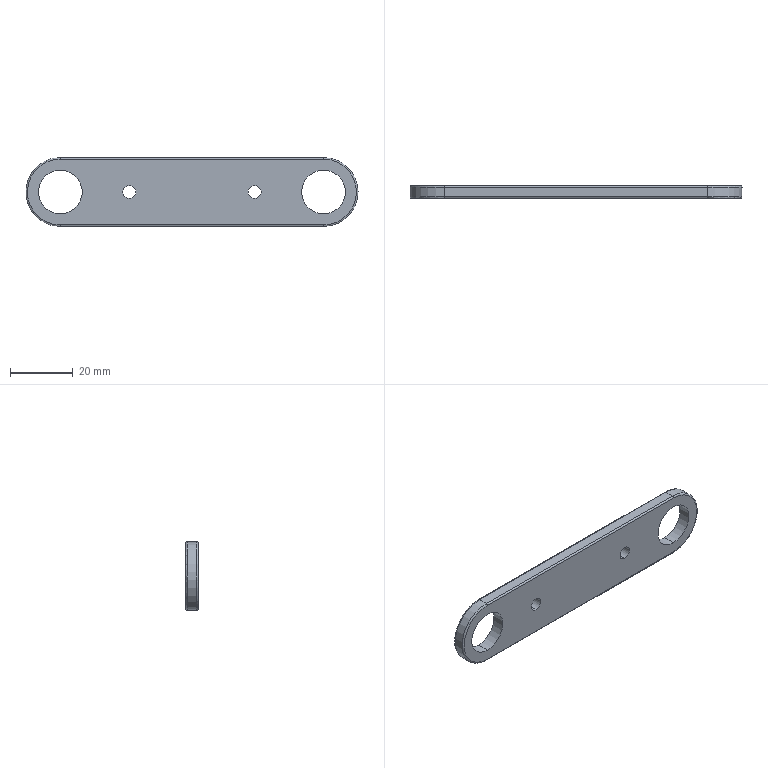Part | SolidWorks | features BaseBody 1 | 1 solid | 23 faces | box 106 x 4 x 22 mm | volume 7550 mm3 | cylinder 15 | plane 4 | spline 4 | commonest cylinder face diameters 1 x4 4.2 x4 13.97 x4 22 x3
STEP:
#1=CARTESIAN_POINT('',(42.,4.,-6.985));
#2=VERTEX_POINT('',#1);
#3=CARTESIAN_POINT('',(42.,4.,6.985));
#4=VERTEX_POINT('',#3);
#5=CARTESIAN_POINT('',(42.,4.,0.));
#6=DIRECTION('',(0.,1.,0.));
#7=DIRECTION('',(0.,0.,-1.));
#8=AXIS2_PLACEMENT_3D('',#5,#6,#7);
#9=CIRCLE('',#8,6.985);
#10=EDGE_CURVE('',#2,#4,#9,.T.);
#11=ORIENTED_EDGE('',*,*,#10,.T.);
#12=CARTESIAN_POINT('',(42.,0.,6.985));
#13=VERTEX_POINT('',#12);
#14=CARTESIAN_POINT('',(42.,4.,6.985));
#15=DIRECTION('',(0.,-1.,0.));
#16=VECTOR('',#15,1000.);
#17=LINE('',#14,#16);
#18=EDGE_CURVE('',#4,#13,#17,.T.);
#19=ORIENTED_EDGE('',*,*,#18,.T.);
#20=CARTESIAN_POINT('',(42.,0.,-6.985));
#21=VERTEX_POINT('',#20);
#22=CARTESIAN_POINT('',(42.,0.,0.));
#23=DIRECTION('',(0.,-1.,0.));
#24=DIRECTION('',(0.,0.,-1.));
#25=AXIS2_PLACEMENT_3D('',#22,#23,#24);
#26=CIRCLE('',#25,6.985);
#27=EDGE_CURVE('',#13,#21,#26,.T.);
#28=ORIENTED_EDGE('',*,*,#27,.T.);
#29=CARTESIAN_POINT('',(42.,4.,-6.985));
#30=DIRECTION('',(0.,-1.,0.));
#31=VECTOR('',#30,1000.);
#32=LINE('',#29,#31);
#33=EDGE_CURVE('',#2,#21,#32,.T.);
#34=ORIENTED_EDGE('',*,*,#33,.F.);
#35=EDGE_LOOP('',(#11,#19,#28,#34));
#36=FACE_OUTER_BOUND('',#35,.T.);
#37=CARTESIAN_POINT('',(42.,4.,0.));
#38=DIRECTION('',(0.,-1.,0.));
#39=DIRECTION('',(0.,0.,-1.));
#40=AXIS2_PLACEMENT_3D('',#37,#38,#39);
#41=CYLINDRICAL_SURFACE('',#40,6.985);
#42=ADVANCED_FACE('',(#36),#41,.F.);
#43=CARTESIAN_POINT('',(-42.,4.,6.985));
#44=VERTEX_POINT('',#43);
#45=CARTESIAN_POINT('',(-42.,4.,-6.985));
#46=VERTEX_POINT('',#45);
#47=CARTESIAN_POINT('',(-42.,4.,0.));
#48=DIRECTION('',(0.,-1.,0.));
#49=DIRECTION('',(0.,0.,-1.));
#50=AXIS2_PLACEMENT_3D('',#47,#48,#49);
#51=CIRCLE('',#50,6.985);
#52=EDGE_CURVE('',#44,#46,#51,.T.);
#53=ORIENTED_EDGE('',*,*,#52,.F.);
#54=CARTESIAN_POINT('',(-42.,0.,6.985));
#55=VERTEX_POINT('',#54);
#56=CARTESIAN_POINT('',(-42.,4.,6.985));
#57=DIRECTION('',(0.,-1.,0.));
#58=VECTOR('',#57,1000.);
#59=LINE('',#56,#58);
#60=EDGE_CURVE('',#44,#55,#59,.T.);
#61=ORIENTED_EDGE('',*,*,#60,.T.);
#62=CARTESIAN_POINT('',(-42.,0.,-6.985));
#63=VERTEX_POINT('',#62);
#64=CARTESIAN_POINT('',(-42.,0.,0.));
#65=DIRECTION('',(0.,-1.,0.));
#66=DIRECTION('',(0.,0.,-1.));
#67=AXIS2_PLACEMENT_3D('',#64,#65,#66);
#68=CIRCLE('',#67,6.985);
#69=EDGE_CURVE('',#55,#63,#68,.T.);
#70=ORIENTED_EDGE('',*,*,#69,.T.);
#71=CARTESIAN_POINT('',(-42.,4.,-6.985));
#72=DIRECTION('',(0.,-1.,0.));
#73=VECTOR('',#72,1000.);
#74=LINE('',#71,#73);
#75=EDGE_CURVE('',#46,#63,#74,.T.);
#76=ORIENTED_EDGE('',*,*,#75,.F.);
#77=EDGE_LOOP('',(#53,#61,#70,#76));
#78=FACE_OUTER_BOUND('',#77,.T.);
#79=CARTESIAN_POINT('',(-42.,4.,0.));
#80=DIRECTION('',(0.,-1.,0.));
#81=DIRECTION('',(0.,0.,-1.));
#82=AXIS2_PLACEMENT_3D('',#79,#80,#81);
#83=CYLINDRICAL_SURFACE('',#82,6.985);
#84=ADVANCED_FACE('',(#78),#83,.F.);
#85=CARTESIAN_POINT('',(-20.,4.,2.1));
#86=VERTEX_POINT('',#85);
#87=CARTESIAN_POINT('',(-20.,4.,-2.1));
#88=VERTEX_POINT('',#87);
#89=CARTESIAN_POINT('',(-20.,4.,0.));
#90=DIRECTION('',(0.,-1.,0.));
#91=DIRECTION('',(0.,0.,-1.));
#92=AXIS2_PLACEMENT_3D('',#89,#90,#91);
#93=CIRCLE('',#92,2.1);
#94=EDGE_CURVE('',#86,#88,#93,.T.);
#95=ORIENTED_EDGE('',*,*,#94,.F.);
#96=CARTESIAN_POINT('',(-20.,0.,2.1));
#97=VERTEX_POINT('',#96);
#98=CARTESIAN_POINT('',(-20.,4.,2.1));
#99=DIRECTION('',(0.,-1.,0.));
#100=VECTOR('',#99,1000.);
#101=LINE('',#98,#100);
#102=EDGE_CURVE('',#86,#97,#101,.T.);
#103=ORIENTED_EDGE('',*,*,#102,.T.);
#104=CARTESIAN_POINT('',(-20.,0.,-2.1));
#105=VERTEX_POINT('',#104);
#106=CARTESIAN_POINT('',(-20.,0.,0.));
#107=DIRECTION('',(0.,-1.,0.));
#108=DIRECTION('',(0.,0.,-1.));
#109=AXIS2_PLACEMENT_3D('',#106,#107,#108);
#110=CIRCLE('',#109,2.1);
#111=EDGE_CURVE('',#97,#105,#110,.T.);
#112=ORIENTED_EDGE('',*,*,#111,.T.);
#113=CARTESIAN_POINT('',(-20.,4.,-2.1));
#114=DIRECTION('',(0.,-1.,0.));
#115=VECTOR('',#114,1000.);
#116=LINE('',#113,#115);
#117=EDGE_CURVE('',#88,#105,#116,.T.);
#118=ORIENTED_EDGE('',*,*,#117,.F.);
#119=EDGE_LOOP('',(#95,#103,#112,#118));
#120=FACE_OUTER_BOUND('',#119,.T.);
#121=CARTESIAN_POINT('',(-20.,4.,0.));
#122=DIRECTION('',(0.,-1.,0.));
#123=DIRECTION('',(0.,0.,-1.));
#124=AXIS2_PLACEMENT_3D('',#121,#122,#123);
#125=CYLINDRICAL_SURFACE('',#124,2.1);
#126=ADVANCED_FACE('',(#120),#125,.F.);
#127=CARTESIAN_POINT('',(20.,4.,2.1));
#128=VERTEX_POINT('',#127);
#129=CARTESIAN_POINT('',(20.,4.,-2.1));
#130=VERTEX_POINT('',#129);
#131=CARTESIAN_POINT('',(20.,4.,0.));
#132=DIRECTION('',(0.,-1.,0.));
#133=DIRECTION('',(0.,0.,-1.));
#134=AXIS2_PLACEMENT_3D('',#131,#132,#133);
#135=CIRCLE('',#134,2.1);
#136=EDGE_CURVE('',#128,#130,#135,.T.);
#137=ORIENTED_EDGE('',*,*,#136,.F.);
#138=CARTESIAN_POINT('',(20.,0.,2.1));
#139=VERTEX_POINT('',#138);
#140=CARTESIAN_POINT('',(20.,4.,2.1));
#141=DIRECTION('',(0.,-1.,0.));
#142=VECTOR('',#141,1000.);
#143=LINE('',#140,#142);
#144=EDGE_CURVE('',#128,#139,#143,.T.);
#145=ORIENTED_EDGE('',*,*,#144,.T.);
#146=CARTESIAN_POINT('',(20.,0.,-2.1));
#147=VERTEX_POINT('',#146);
#148=CARTESIAN_POINT('',(20.,0.,0.));
#149=DIRECTION('',(0.,-1.,0.));
#150=DIRECTION('',(0.,0.,-1.));
#151=AXIS2_PLACEMENT_3D('',#148,#149,#150);
#152=CIRCLE('',#151,2.1);
#153=EDGE_CURVE('',#139,#147,#152,.T.);
#154=ORIENTED_EDGE('',*,*,#153,.T.);
#155=CARTESIAN_POINT('',(20.,4.,-2.1));
#156=DIRECTION('',(0.,-1.,0.));
#157=VECTOR('',#156,1000.);
#158=LINE('',#155,#157);
#159=EDGE_CURVE('',#130,#147,#158,.T.);
#160=ORIENTED_EDGE('',*,*,#159,.F.);
#161=EDGE_LOOP('',(#137,#145,#154,#160));
#162=FACE_OUTER_BOUND('',#161,.T.);
#163=CARTESIAN_POINT('',(20.,4.,0.));
#164=DIRECTION('',(0.,-1.,0.));
#165=DIRECTION('',(0.,0.,-1.));
#166=AXIS2_PLACEMENT_3D('',#163,#164,#165);
#167=CYLINDRICAL_SURFACE('',#166,2.1);
#168=ADVANCED_FACE('',(#162),#167,.F.);
#169=CARTESIAN_POINT('',(53.,3.5,0.));
#170=VERTEX_POINT('',#169);
#171=CARTESIAN_POINT('',(42.,3.5,-11.));
#172=VERTEX_POINT('',#171);
#173=CARTESIAN_POINT('',(42.,3.5,0.));
#174=DIRECTION('',(0.,1.,0.));
#175=DIRECTION('',(0.,0.,1.));
#176=AXIS2_PLACEMENT_3D('',#173,#174,#175);
#177=CIRCLE('',#176,11.);
#178=EDGE_CURVE('',#170,#172,#177,.T.);
#179=ORIENTED_EDGE('',*,*,#178,.F.);
#180=CARTESIAN_POINT('',(53.,0.5,0.));
#181=VERTEX_POINT('',#180);
#182=CARTESIAN_POINT('',(53.,3.5,0.));
#183=DIRECTION('',(0.,-1.,0.));
#184=VECTOR('',#183,1000.);
#185=LINE('',#182,#184);
#186=EDGE_CURVE('',#170,#181,#185,.T.);
#187=ORIENTED_EDGE('',*,*,#186,.T.);
#188=CARTESIAN_POINT('',(42.,0.5,-11.));
#189=VERTEX_POINT('',#188);
#190=CARTESIAN_POINT('',(42.,0.5,0.));
#191=DIRECTION('',(0.,-1.,0.));
#192=DIRECTION('',(0.,0.,-1.));
#193=AXIS2_PLACEMENT_3D('',#190,#191,#192);
#194=CIRCLE('',#193,11.);
#195=EDGE_CURVE('',#189,#181,#194,.T.);
#196=ORIENTED_EDGE('',*,*,#195,.F.);
#197=CARTESIAN_POINT('',(42.,2.,-11.));
#198=DIRECTION('',(0.,1.,0.));
#199=VECTOR('',#198,1000.);
#200=LINE('',#197,#199);
#201=EDGE_CURVE('',#189,#172,#200,.T.);
#202=ORIENTED_EDGE('',*,*,#201,.T.);
#203=EDGE_LOOP('',(#179,#187,#196,#202));
#204=FACE_OUTER_BOUND('',#203,.T.);
#205=CARTESIAN_POINT('',(42.,3.5,0.));
#206=DIRECTION('',(0.,-1.,0.));
#207=DIRECTION('',(1.,0.,0.));
#208=AXIS2_PLACEMENT_3D('',#205,#206,#207);
#209=CYLINDRICAL_SURFACE('',#208,11.);
#210=ADVANCED_FACE('',(#204),#209,.T.);
#211=ORIENTED_EDGE('',*,*,#18,.F.);
#212=CARTESIAN_POINT('',(42.,4.,0.));
#213=DIRECTION('',(0.,1.,0.));
#214=DIRECTION('',(0.,0.,-1.));
#215=AXIS2_PLACEMENT_3D('',#212,#213,#214);
#216=CIRCLE('',#215,6.985);
#217=EDGE_CURVE('',#4,#2,#216,.T.);
#218=ORIENTED_EDGE('',*,*,#217,.T.);
#219=ORIENTED_EDGE('',*,*,#33,.T.);
#220=CARTESIAN_POINT('',(42.,0.,0.));
#221=DIRECTION('',(0.,-1.,0.));
#222=DIRECTION('',(0.,0.,-1.));
#223=AXIS2_PLACEMENT_3D('',#220,#221,#222);
#224=CIRCLE('',#223,6.985);
#225=EDGE_CURVE('',#21,#13,#224,.T.);
#226=ORIENTED_EDGE('',*,*,#225,.T.);
#227=EDGE_LOOP('',(#211,#218,#219,#226));
#228=FACE_OUTER_BOUND('',#227,.T.);
#229=CARTESIAN_POINT('',(42.,4.,0.));
#230=DIRECTION('',(0.,-1.,0.));
#231=DIRECTION('',(0.,0.,-1.));
#232=AXIS2_PLACEMENT_3D('',#229,#230,#231);
#233=CYLINDRICAL_SURFACE('',#232,6.985);
#234=ADVANCED_FACE('',(#228),#233,.F.);
#235=ORIENTED_EDGE('',*,*,#225,.F.);
#236=ORIENTED_EDGE('',*,*,#27,.F.);
#237=EDGE_LOOP('',(#235,#236));
#238=FACE_BOUND('',#237,.T.);
#239=CARTESIAN_POINT('',(-42.,0.,0.));
#240=DIRECTION('',(0.,-1.,0.));
#241=DIRECTION('',(0.,0.,-1.));
#242=AXIS2_PLACEMENT_3D('',#239,#240,#241);
#243=CIRCLE('',#242,6.985);
#244=EDGE_CURVE('',#63,#55,#243,.T.);
#245=ORIENTED_EDGE('',*,*,#244,.F.);
#246=ORIENTED_EDGE('',*,*,#69,.F.);
#247=EDGE_LOOP('',(#245,#246));
#248=FACE_BOUND('',#247,.T.);
#249=CARTESIAN_POINT('',(-20.,0.,0.));
#250=DIRECTION('',(0.,-1.,0.));
#251=DIRECTION('',(0.,0.,-1.));
#252=AXIS2_PLACEMENT_3D('',#249,#250,#251);
#253=CIRCLE('',#252,2.1);
#254=EDGE_CURVE('',#105,#97,#253,.T.);
#255=ORIENTED_EDGE('',*,*,#254,.F.);
#256=ORIENTED_EDGE('',*,*,#111,.F.);
#257=EDGE_LOOP('',(#255,#256));
#258=FACE_BOUND('',#257,.T.);
#259=CARTESIAN_POINT('',(20.,0.,0.));
#260=DIRECTION('',(0.,-1.,0.));
#261=DIRECTION('',(0.,0.,-1.));
#262=AXIS2_PLACEMENT_3D('',#259,#260,#261);
#263=CIRCLE('',#262,2.1);
#264=EDGE_CURVE('',#147,#139,#263,.T.);
#265=ORIENTED_EDGE('',*,*,#264,.F.);
#266=ORIENTED_EDGE('',*,*,#153,.F.);
#267=EDGE_LOOP('',(#265,#266));
#268=FACE_BOUND('',#267,.T.);
#269=CARTESIAN_POINT('',(-42.,0.,-10.5));
#270=VERTEX_POINT('',#269);
#271=CARTESIAN_POINT('',(-42.,0.,10.5));
#272=VERTEX_POINT('',#271);
#273=CARTESIAN_POINT('',(-42.,0.,-10.5));
#274=CARTESIAN_POINT('',(-63.,0.,-10.5));
#275=CARTESIAN_POINT('',(-63.,0.,10.5));
#276=CARTESIAN_POINT('',(-42.,0.,10.5));
#277=(BOUNDED_CURVE()B_SPLINE_CURVE(3,(#273,#274,#275,#276),.UNSPECIFIED.,.F.,.T.)B_SPLINE_CURVE_WITH_KNOTS((4,4),(0.,1.),.UNSPECIFIED.)CURVE()GEOMETRIC_REPRESENTATION_ITEM()RATIONAL_B_SPLINE_CURVE((0.9566,0.3189,0.3189,0.9566))REPRESENTATION_ITEM(''));
#278=EDGE_CURVE('',#270,#272,#277,.T.);
#279=ORIENTED_EDGE('',*,*,#278,.F.);
#280=CARTESIAN_POINT('',(42.,0.,-10.5));
#281=VERTEX_POINT('',#280);
#282=CARTESIAN_POINT('',(0.,0.,-10.5));
#283=DIRECTION('',(-1.,0.,0.));
#284=VECTOR('',#283,1000.);
#285=LINE('',#282,#284);
#286=EDGE_CURVE('',#281,#270,#285,.T.);
#287=ORIENTED_EDGE('',*,*,#286,.F.);
#288=CARTESIAN_POINT('',(42.,0.,10.5));
#289=VERTEX_POINT('',#288);
#290=CARTESIAN_POINT('',(42.,0.,10.5));
#291=CARTESIAN_POINT('',(63.,0.,10.5));
#292=CARTESIAN_POINT('',(63.,0.,-10.5));
#293=CARTESIAN_POINT('',(42.,0.,-10.5));
#294=(BOUNDED_CURVE()B_SPLINE_CURVE(3,(#290,#291,#292,#293),.UNSPECIFIED.,.F.,.F.)B_SPLINE_CURVE_WITH_KNOTS((4,4),(0.,1.),.UNSPECIFIED.)CURVE()GEOMETRIC_REPRESENTATION_ITEM()RATIONAL_B_SPLINE_CURVE((0.9566,0.3189,0.3189,0.9566))REPRESENTATION_ITEM(''));
#295=EDGE_CURVE('',#289,#281,#294,.T.);
#296=ORIENTED_EDGE('',*,*,#295,.F.);
#297=CARTESIAN_POINT('',(0.,0.,10.5));
#298=DIRECTION('',(1.,0.,0.));
#299=VECTOR('',#298,1000.);
#300=LINE('',#297,#299);
#301=EDGE_CURVE('',#272,#289,#300,.T.);
#302=ORIENTED_EDGE('',*,*,#301,.F.);
#303=EDGE_LOOP('',(#279,#287,#296,#302));
#304=FACE_OUTER_BOUND('',#303,.T.);
#305=CARTESIAN_POINT('',(-53.13,0.,-10.5));
#306=DIRECTION('',(0.,1.,0.));
#307=DIRECTION('',(0.,0.,1.));
#308=AXIS2_PLACEMENT_3D('',#305,#306,#307);
#309=PLANE('',#308);
#310=ADVANCED_FACE('',(#238,#248,#258,#268,#304),#309,.F.);
#311=ORIENTED_EDGE('',*,*,#10,.F.);
#312=ORIENTED_EDGE('',*,*,#217,.F.);
#313=EDGE_LOOP('',(#311,#312));
#314=FACE_BOUND('',#313,.T.);
#315=CARTESIAN_POINT('',(-42.,4.,0.));
#316=DIRECTION('',(0.,-1.,0.));
#317=DIRECTION('',(0.,0.,-1.));
#318=AXIS2_PLACEMENT_3D('',#315,#316,#317);
#319=CIRCLE('',#318,6.985);
#320=EDGE_CURVE('',#46,#44,#319,.T.);
#321=ORIENTED_EDGE('',*,*,#320,.T.);
#322=ORIENTED_EDGE('',*,*,#52,.T.);
#323=EDGE_LOOP('',(#321,#322));
#324=FACE_BOUND('',#323,.T.);
#325=CARTESIAN_POINT('',(-20.,4.,0.));
#326=DIRECTION('',(0.,-1.,0.));
#327=DIRECTION('',(0.,0.,-1.));
#328=AXIS2_PLACEMENT_3D('',#325,#326,#327);
#329=CIRCLE('',#328,2.1);
#330=EDGE_CURVE('',#88,#86,#329,.T.);
#331=ORIENTED_EDGE('',*,*,#330,.T.);
#332=ORIENTED_EDGE('',*,*,#94,.T.);
#333=EDGE_LOOP('',(#331,#332));
#334=FACE_BOUND('',#333,.T.);
#335=CARTESIAN_POINT('',(20.,4.,0.));
#336=DIRECTION('',(0.,-1.,0.));
#337=DIRECTION('',(0.,0.,-1.));
#338=AXIS2_PLACEMENT_3D('',#335,#336,#337);
#339=CIRCLE('',#338,2.1);
#340=EDGE_CURVE('',#130,#128,#339,.T.);
#341=ORIENTED_EDGE('',*,*,#340,.T.);
#342=ORIENTED_EDGE('',*,*,#136,.T.);
#343=EDGE_LOOP('',(#341,#342));
#344=FACE_BOUND('',#343,.T.);
#345=CARTESIAN_POINT('',(-42.,4.,10.5));
#346=VERTEX_POINT('',#345);
#347=CARTESIAN_POINT('',(42.,4.,10.5));
#348=VERTEX_POINT('',#347);
#349=CARTESIAN_POINT('',(0.,4.,10.5));
#350=DIRECTION('',(1.,0.,0.));
#351=VECTOR('',#350,1000.);
#352=LINE('',#349,#351);
#353=EDGE_CURVE('',#346,#348,#352,.T.);
#354=ORIENTED_EDGE('',*,*,#353,.T.);
#355=CARTESIAN_POINT('',(42.,4.,-10.5));
#356=VERTEX_POINT('',#355);
#357=CARTESIAN_POINT('',(42.,4.,10.5));
#358=CARTESIAN_POINT('',(42.233,4.,10.5));
#359=CARTESIAN_POINT('',(42.583,4.,10.488));
#360=CARTESIAN_POINT('',(42.989,4.,10.454));
#361=CARTESIAN_POINT('',(43.191,4.,10.432));
#362=CARTESIAN_POINT('',(43.293,4.,10.42));
#363=CARTESIAN_POINT('',(43.336,4.,10.415));
#364=CARTESIAN_POINT('',(43.365,4.,10.411));
#365=CARTESIAN_POINT('',(43.377,4.,10.409));
#366=CARTESIAN_POINT('',(43.655,4.,10.372));
#367=CARTESIAN_POINT('',(44.045,4.,10.305));
#368=CARTESIAN_POINT('',(44.494,4.,10.201));
#369=CARTESIAN_POINT('',(44.718,4.,10.143));
#370=CARTESIAN_POINT('',(44.829,4.,10.112));
#371=CARTESIAN_POINT('',(44.877,4.,10.098));
#372=CARTESIAN_POINT('',(44.908,4.,10.089));
#373=CARTESIAN_POINT('',(44.922,4.,10.085));
#374=CARTESIAN_POINT('',(45.226,4.,9.997));
#375=CARTESIAN_POINT('',(45.648,4.,9.854));
#376=CARTESIAN_POINT('',(46.128,4.,9.656));
#377=CARTESIAN_POINT('',(46.366,4.,9.55));
#378=CARTESIAN_POINT('',(46.484,4.,9.495));
#379=CARTESIAN_POINT('',(46.534,4.,9.471));
#380=CARTESIAN_POINT('',(46.568,4.,9.454));
#381=CARTESIAN_POINT('',(46.582,4.,9.447));
#382=CARTESIAN_POINT('',(46.901,4.,9.292));
#383=CARTESIAN_POINT('',(47.338,4.,9.053));
#384=CARTESIAN_POINT('',(47.826,4.,8.738));
#385=CARTESIAN_POINT('',(48.065,4.,8.572));
#386=CARTESIAN_POINT('',(48.183,4.,8.487));
#387=CARTESIAN_POINT('',(48.233,4.,8.45));
#388=CARTESIAN_POINT('',(48.267,4.,8.425));
#389=CARTESIAN_POINT('',(48.282,4.,8.414));
#390=CARTESIAN_POINT('',(48.595,4.,8.179));
#391=CARTESIAN_POINT('',(49.017,4.,7.826));
#392=CARTESIAN_POINT('',(49.475,4.,7.378));
#393=CARTESIAN_POINT('',(49.696,4.,7.144));
#394=CARTESIAN_POINT('',(49.804,4.,7.025));
#395=CARTESIAN_POINT('',(49.85,4.,6.973));
#396=CARTESIAN_POINT('',(49.881,4.,6.939));
#397=CARTESIAN_POINT('',(49.895,4.,6.923));
#398=CARTESIAN_POINT('',(50.04,4.,6.757));
#399=CARTESIAN_POINT('',(50.226,4.,6.53));
#400=CARTESIAN_POINT('',(50.433,4.,6.258));
#401=CARTESIAN_POINT('',(50.519,4.,6.139));
#402=CARTESIAN_POINT('',(50.576,4.,6.059));
#403=CARTESIAN_POINT('',(50.603,4.,6.02));
#404=CARTESIAN_POINT('',(50.747,4.,5.812));
#405=CARTESIAN_POINT('',(50.913,4.,5.557));
#406=CARTESIAN_POINT('',(51.093,4.,5.252));
#407=CARTESIAN_POINT('',(51.168,4.,5.119));
#408=CARTESIAN_POINT('',(51.217,4.,5.031));
#409=CARTESIAN_POINT('',(51.24,4.,4.987));
#410=CARTESIAN_POINT('',(51.363,4.,4.757));
#411=CARTESIAN_POINT('',(51.502,4.,4.477));
#412=CARTESIAN_POINT('',(51.628,4.,4.19));
#413=CARTESIAN_POINT('',(51.71,4.,3.998));
#414=CARTESIAN_POINT('',(51.748,4.,3.903));
#415=CARTESIAN_POINT('',(51.864,4.,3.605));
#416=CARTESIAN_POINT('',(51.971,4.,3.303));
#417=CARTESIAN_POINT('',(52.064,4.,2.997));
#418=CARTESIAN_POINT('',(52.123,4.,2.791));
#419=CARTESIAN_POINT('',(52.15,4.,2.69));
#420=CARTESIAN_POINT('',(52.23,4.,2.374));
#421=CARTESIAN_POINT('',(52.277,4.,2.163));
#422=CARTESIAN_POINT('',(52.358,4.,1.737));
#423=CARTESIAN_POINT('',(52.391,4.,1.524));
#424=CARTESIAN_POINT('',(52.473,4.,0.8737));
#425=CARTESIAN_POINT('',(52.5,4.,0.4371));
#426=CARTESIAN_POINT('',(52.5,4.,-0.2186));
#427=CARTESIAN_POINT('',(52.493,4.,-0.4368));
#428=CARTESIAN_POINT('',(52.466,4.,-0.8726));
#429=CARTESIAN_POINT('',(52.445,4.,-1.092));
#430=CARTESIAN_POINT('',(52.391,4.,-1.523));
#431=CARTESIAN_POINT('',(52.341,4.,-1.844));
#432=CARTESIAN_POINT('',(52.276,4.,-2.162));
#433=CARTESIAN_POINT('',(52.229,4.,-2.374));
#434=CARTESIAN_POINT('',(52.203,4.,-2.481));
#435=CARTESIAN_POINT('',(52.124,4.,-2.792));
#436=CARTESIAN_POINT('',(52.036,4.,-3.099));
#437=CARTESIAN_POINT('',(51.917,4.,-3.453));
#438=CARTESIAN_POINT('',(51.862,4.,-3.604));
#439=CARTESIAN_POINT('',(51.825,4.,-3.704));
#440=CARTESIAN_POINT('',(51.806,4.,-3.755));
#441=CARTESIAN_POINT('',(51.711,4.,-3.998));
#442=CARTESIAN_POINT('',(51.589,4.,-4.287));
#443=CARTESIAN_POINT('',(51.432,4.,-4.616));
#444=CARTESIAN_POINT('',(51.361,4.,-4.756));
#445=CARTESIAN_POINT('',(51.314,4.,-4.849));
#446=CARTESIAN_POINT('',(51.289,4.,-4.896));
#447=CARTESIAN_POINT('',(51.169,4.,-5.12));
#448=CARTESIAN_POINT('',(51.019,4.,-5.384));
#449=CARTESIAN_POINT('',(50.83,4.,-5.684));
#450=CARTESIAN_POINT('',(50.746,4.,-5.811));
#451=CARTESIAN_POINT('',(50.689,4.,-5.895));
#452=CARTESIAN_POINT('',(50.66,4.,-5.938));
#453=CARTESIAN_POINT('',(50.52,4.,-6.139));
#454=CARTESIAN_POINT('',(50.347,4.,-6.376));
#455=CARTESIAN_POINT('',(50.133,4.,-6.643));
#456=CARTESIAN_POINT('',(50.023,4.,-6.774));
#457=CARTESIAN_POINT('',(49.975,4.,-6.83));
#458=CARTESIAN_POINT('',(49.943,4.,-6.867));
#459=CARTESIAN_POINT('',(49.926,4.,-6.887));
#460=CARTESIAN_POINT('',(49.669,4.,-7.182));
#461=CARTESIAN_POINT('',(49.286,4.,-7.577));
#462=CARTESIAN_POINT('',(48.804,4.,-8.001));
#463=CARTESIAN_POINT('',(48.555,4.,-8.203));
#464=CARTESIAN_POINT('',(48.428,4.,-8.302));
#465=CARTESIAN_POINT('',(48.373,4.,-8.344));
#466=CARTESIAN_POINT('',(48.337,4.,-8.372));
#467=CARTESIAN_POINT('',(48.317,4.,-8.388));
#468=CARTESIAN_POINT('',(48.033,4.,-8.6));
#469=CARTESIAN_POINT('',(47.621,4.,-8.88));
#470=CARTESIAN_POINT('',(47.118,4.,-9.171));
#471=CARTESIAN_POINT('',(46.862,4.,-9.307));
#472=CARTESIAN_POINT('',(46.732,4.,-9.374));
#473=CARTESIAN_POINT('',(46.676,4.,-9.401));
#474=CARTESIAN_POINT('',(46.639,4.,-9.42));
#475=CARTESIAN_POINT('',(46.618,4.,-9.43));
#476=CARTESIAN_POINT('',(46.334,4.,-9.569));
#477=CARTESIAN_POINT('',(45.925,4.,-9.747));
#478=CARTESIAN_POINT('',(45.437,4.,-9.924));
#479=CARTESIAN_POINT('',(45.189,4.,-10.004));
#480=CARTESIAN_POINT('',(45.065,4.,-10.043));
#481=CARTESIAN_POINT('',(45.011,4.,-10.059));
#482=CARTESIAN_POINT('',(44.976,4.,-10.07));
#483=CARTESIAN_POINT('',(44.956,4.,-10.075));
#484=CARTESIAN_POINT('',(44.687,4.,-10.154));
#485=CARTESIAN_POINT('',(44.303,4.,-10.25));
#486=CARTESIAN_POINT('',(43.85,4.,-10.337));
#487=CARTESIAN_POINT('',(43.623,4.,-10.374));
#488=CARTESIAN_POINT('',(43.508,4.,-10.391));
#489=CARTESIAN_POINT('',(43.459,4.,-10.398));
#490=CARTESIAN_POINT('',(43.427,4.,-10.403));
#491=CARTESIAN_POINT('',(43.408,4.,-10.405));
#492=CARTESIAN_POINT('',(42.932,4.,-10.469));
#493=CARTESIAN_POINT('',(42.467,4.,-10.5));
#494=CARTESIAN_POINT('',(42.,4.,-10.5));
#495=B_SPLINE_CURVE_WITH_KNOTS('',3,(#357,#358,#359,#360,#361,#362,#363,#364,#365,#366,#367,#368,#369,#370,#371,#372,#373,#374,#375,#376,#377,#378,#379,#380,#381,#382,#383,#384,#385,#386,#387,#388,#389,#390,#391,#392,#393,#394,#395,#396,#397,#398,#399,#400,#401,#402,#403,#404,#405,#406,#407,#408,#409,#410,#411,#412,#413,#414,#415,#416,#417,#418,#419,#420,#421,#422,#423,#424,#425,#426,#427,#428,#429,#430,#431,#432,#433,#434,#435,#436,#437,#438,#439,#440,#441,#442,#443,#444,#445,#446,#447,#448,#449,#450,#451,#452,#453,#454,#455,#456,#457,#458,#459,#460,#461,#462,#463,#464,#465,#466,#467,#468,#469,#470,#471,#472,#473,#474,#475,#476,#477,#478,#479,#480,#481,#482,#483,#484,#485,#486,#487,#488,#489,#490,#491,#492,#493,#494),.UNSPECIFIED.,.F.,.F.,(4,1,1,1,1,2,2,1,1,1,1,2,2,1,1,1,1,2,2,1,1,1,1,2,2,1,1,1,1,2,2,1,1,2,2,1,1,2,2,1,2,2,1,2,2,2,2,2,2,2,1,2,2,1,1,2,2,1,1,2,2,1,1,2,2,1,1,1,2,2,1,1,1,1,2,2,1,1,1,1,2,2,1,1,1,1,2,2,1,1,1,1,2,2,4),(0.,0.03125,0.04688,0.05469,0.05859,0.06055,0.0625,0.09375,0.1094,0.1172,0.1211,0.123,0.125,0.1563,0.1719,0.1797,0.1836,0.1855,0.1875,0.2188,0.2344,0.2422,0.2461,0.248,0.25,0.2813,0.2969,0.3047,0.3086,0.3105,0.3125,0.3281,0.3359,0.3398,0.3438,0.3594,0.3672,0.3711,0.375,0.3906,0.3984,0.4063,0.4219,0.4297,0.4375,0.4531,0.4688,0.5,0.5156,0.5313,0.5469,0.5547,0.5625,0.5781,0.5859,0.5898,0.5938,0.6094,0.6172,0.6211,0.625,0.6406,0.6484,0.6523,0.6562,0.6719,0.6797,0.6836,0.6855,0.6875,0.7187,0.7344,0.7422,0.7461,0.748,0.75,0.7812,0.7969,0.8047,0.8086,0.8105,0.8125,0.8437,0.8594,0.8672,0.8711,0.873,0.875,0.9062,0.9219,0.9297,0.9336,0.9355,0.9375,1.),.UNSPECIFIED.);
#496=EDGE_CURVE('',#348,#356,#495,.T.);
#497=ORIENTED_EDGE('',*,*,#496,.T.);
#498=CARTESIAN_POINT('',(-42.,4.,-10.5));
#499=VERTEX_POINT('',#498);
#500=CARTESIAN_POINT('',(0.,4.,-10.5));
#501=DIRECTION('',(-1.,0.,0.));
#502=VECTOR('',#501,1000.);
#503=LINE('',#500,#502);
#504=EDGE_CURVE('',#356,#499,#503,.T.);
#505=ORIENTED_EDGE('',*,*,#504,.T.);
#506=CARTESIAN_POINT('',(-42.,4.,-10.5));
#507=CARTESIAN_POINT('',(-42.233,4.,-10.5));
#508=CARTESIAN_POINT('',(-42.583,4.,-10.488));
#509=CARTESIAN_POINT('',(-42.989,4.,-10.454));
#510=CARTESIAN_POINT('',(-43.191,4.,-10.432));
#511=CARTESIAN_POINT('',(-43.293,4.,-10.42));
#512=CARTESIAN_POINT('',(-43.336,4.,-10.415));
#513=CARTESIAN_POINT('',(-43.365,4.,-10.411));
#514=CARTESIAN_POINT('',(-43.377,4.,-10.409));
#515=CARTESIAN_POINT('',(-43.655,4.,-10.372));
#516=CARTESIAN_POINT('',(-44.045,4.,-10.305));
#517=CARTESIAN_POINT('',(-44.494,4.,-10.201));
#518=CARTESIAN_POINT('',(-44.718,4.,-10.143));
#519=CARTESIAN_POINT('',(-44.829,4.,-10.112));
#520=CARTESIAN_POINT('',(-44.877,4.,-10.098));
#521=CARTESIAN_POINT('',(-44.908,4.,-10.089));
#522=CARTESIAN_POINT('',(-44.922,4.,-10.085));
#523=CARTESIAN_POINT('',(-45.226,4.,-9.997));
#524=CARTESIAN_POINT('',(-45.648,4.,-9.854));
#525=CARTESIAN_POINT('',(-46.128,4.,-9.656));
#526=CARTESIAN_POINT('',(-46.366,4.,-9.55));
#527=CARTESIAN_POINT('',(-46.484,4.,-9.495));
#528=CARTESIAN_POINT('',(-46.534,4.,-9.471));
#529=CARTESIAN_POINT('',(-46.568,4.,-9.454));
#530=CARTESIAN_POINT('',(-46.582,4.,-9.447));
#531=CARTESIAN_POINT('',(-46.901,4.,-9.292));
#532=CARTESIAN_POINT('',(-47.338,4.,-9.053));
#533=CARTESIAN_POINT('',(-47.826,4.,-8.738));
#534=CARTESIAN_POINT('',(-48.065,4.,-8.572));
#535=CARTESIAN_POINT('',(-48.183,4.,-8.487));
#536=CARTESIAN_POINT('',(-48.233,4.,-8.45));
#537=CARTESIAN_POINT('',(-48.267,4.,-8.425));
#538=CARTESIAN_POINT('',(-48.282,4.,-8.414));
#539=CARTESIAN_POINT('',(-48.595,4.,-8.179));
#540=CARTESIAN_POINT('',(-49.017,4.,-7.826));
#541=CARTESIAN_POINT('',(-49.475,4.,-7.378));
#542=CARTESIAN_POINT('',(-49.696,4.,-7.144));
#543=CARTESIAN_POINT('',(-49.804,4.,-7.025));
#544=CARTESIAN_POINT('',(-49.85,4.,-6.973));
#545=CARTESIAN_POINT('',(-49.881,4.,-6.939));
#546=CARTESIAN_POINT('',(-49.895,4.,-6.923));
#547=CARTESIAN_POINT('',(-50.04,4.,-6.757));
#548=CARTESIAN_POINT('',(-50.226,4.,-6.53));
#549=CARTESIAN_POINT('',(-50.433,4.,-6.258));
#550=CARTESIAN_POINT('',(-50.519,4.,-6.139));
#551=CARTESIAN_POINT('',(-50.576,4.,-6.059));
#552=CARTESIAN_POINT('',(-50.603,4.,-6.02));
#553=CARTESIAN_POINT('',(-50.747,4.,-5.812));
#554=CARTESIAN_POINT('',(-50.913,4.,-5.557));
#555=CARTESIAN_POINT('',(-51.093,4.,-5.252));
#556=CARTESIAN_POINT('',(-51.168,4.,-5.119));
#557=CARTESIAN_POINT('',(-51.217,4.,-5.031));
#558=CARTESIAN_POINT('',(-51.24,4.,-4.987));
#559=CARTESIAN_POINT('',(-51.363,4.,-4.757));
#560=CARTESIAN_POINT('',(-51.502,4.,-4.477));
#561=CARTESIAN_POINT('',(-51.628,4.,-4.19));
#562=CARTESIAN_POINT('',(-51.71,4.,-3.998));
#563=CARTESIAN_POINT('',(-51.748,4.,-3.903));
#564=CARTESIAN_POINT('',(-51.864,4.,-3.605));
#565=CARTESIAN_POINT('',(-51.971,4.,-3.303));
#566=CARTESIAN_POINT('',(-52.064,4.,-2.997));
#567=CARTESIAN_POINT('',(-52.123,4.,-2.791));
#568=CARTESIAN_POINT('',(-52.15,4.,-2.69));
#569=CARTESIAN_POINT('',(-52.23,4.,-2.374));
#570=CARTESIAN_POINT('',(-52.277,4.,-2.163));
#571=CARTESIAN_POINT('',(-52.358,4.,-1.737));
#572=CARTESIAN_POINT('',(-52.391,4.,-1.524));
#573=CARTESIAN_POINT('',(-52.473,4.,-0.8737));
#574=CARTESIAN_POINT('',(-52.5,4.,-0.4371));
#575=CARTESIAN_POINT('',(-52.5,4.,0.2186));
#576=CARTESIAN_POINT('',(-52.493,4.,0.4368));
#577=CARTESIAN_POINT('',(-52.466,4.,0.8726));
#578=CARTESIAN_POINT('',(-52.445,4.,1.092));
#579=CARTESIAN_POINT('',(-52.391,4.,1.523));
#580=CARTESIAN_POINT('',(-52.341,4.,1.844));
#581=CARTESIAN_POINT('',(-52.276,4.,2.162));
#582=CARTESIAN_POINT('',(-52.229,4.,2.374));
#583=CARTESIAN_POINT('',(-52.203,4.,2.481));
#584=CARTESIAN_POINT('',(-52.124,4.,2.792));
#585=CARTESIAN_POINT('',(-52.036,4.,3.099));
#586=CARTESIAN_POINT('',(-51.917,4.,3.453));
#587=CARTESIAN_POINT('',(-51.862,4.,3.604));
#588=CARTESIAN_POINT('',(-51.825,4.,3.704));
#589=CARTESIAN_POINT('',(-51.806,4.,3.755));
#590=CARTESIAN_POINT('',(-51.711,4.,3.998));
#591=CARTESIAN_POINT('',(-51.589,4.,4.287));
#592=CARTESIAN_POINT('',(-51.432,4.,4.616));
#593=CARTESIAN_POINT('',(-51.361,4.,4.756));
#594=CARTESIAN_POINT('',(-51.314,4.,4.849));
#595=CARTESIAN_POINT('',(-51.289,4.,4.896));
#596=CARTESIAN_POINT('',(-51.169,4.,5.12));
#597=CARTESIAN_POINT('',(-51.019,4.,5.384));
#598=CARTESIAN_POINT('',(-50.83,4.,5.684));
#599=CARTESIAN_POINT('',(-50.746,4.,5.811));
#600=CARTESIAN_POINT('',(-50.689,4.,5.895));
#601=CARTESIAN_POINT('',(-50.66,4.,5.938));
#602=CARTESIAN_POINT('',(-50.52,4.,6.139));
#603=CARTESIAN_POINT('',(-50.347,4.,6.376));
#604=CARTESIAN_POINT('',(-50.133,4.,6.643));
#605=CARTESIAN_POINT('',(-50.023,4.,6.774));
#606=CARTESIAN_POINT('',(-49.975,4.,6.83));
#607=CARTESIAN_POINT('',(-49.943,4.,6.867));
#608=CARTESIAN_POINT('',(-49.926,4.,6.887));
#609=CARTESIAN_POINT('',(-49.669,4.,7.182));
#610=CARTESIAN_POINT('',(-49.286,4.,7.577));
#611=CARTESIAN_POINT('',(-48.804,4.,8.001));
#612=CARTESIAN_POINT('',(-48.555,4.,8.203));
#613=CARTESIAN_POINT('',(-48.428,4.,8.302));
#614=CARTESIAN_POINT('',(-48.373,4.,8.344));
#615=CARTESIAN_POINT('',(-48.337,4.,8.372));
#616=CARTESIAN_POINT('',(-48.317,4.,8.388));
#617=CARTESIAN_POINT('',(-48.033,4.,8.6));
#618=CARTESIAN_POINT('',(-47.621,4.,8.88));
#619=CARTESIAN_POINT('',(-47.118,4.,9.171));
#620=CARTESIAN_POINT('',(-46.862,4.,9.307));
#621=CARTESIAN_POINT('',(-46.732,4.,9.374));
#622=CARTESIAN_POINT('',(-46.676,4.,9.401));
#623=CARTESIAN_POINT('',(-46.639,4.,9.42));
#624=CARTESIAN_POINT('',(-46.618,4.,9.43));
#625=CARTESIAN_POINT('',(-46.334,4.,9.569));
#626=CARTESIAN_POINT('',(-45.925,4.,9.747));
#627=CARTESIAN_POINT('',(-45.437,4.,9.924));
#628=CARTESIAN_POINT('',(-45.189,4.,10.004));
#629=CARTESIAN_POINT('',(-45.065,4.,10.043));
#630=CARTESIAN_POINT('',(-45.011,4.,10.059));
#631=CARTESIAN_POINT('',(-44.976,4.,10.07));
#632=CARTESIAN_POINT('',(-44.956,4.,10.075));
#633=CARTESIAN_POINT('',(-44.687,4.,10.154));
#634=CARTESIAN_POINT('',(-44.303,4.,10.25));
#635=CARTESIAN_POINT('',(-43.85,4.,10.337));
#636=CARTESIAN_POINT('',(-43.623,4.,10.374));
#637=CARTESIAN_POINT('',(-43.508,4.,10.391));
#638=CARTESIAN_POINT('',(-43.459,4.,10.398));
#639=CARTESIAN_POINT('',(-43.427,4.,10.403));
#640=CARTESIAN_POINT('',(-43.408,4.,10.405));
#641=CARTESIAN_POINT('',(-42.932,4.,10.469));
#642=CARTESIAN_POINT('',(-42.467,4.,10.5));
#643=CARTESIAN_POINT('',(-42.,4.,10.5));
#644=B_SPLINE_CURVE_WITH_KNOTS('',3,(#506,#507,#508,#509,#510,#511,#512,#513,#514,#515,#516,#517,#518,#519,#520,#521,#522,#523,#524,#525,#526,#527,#528,#529,#530,#531,#532,#533,#534,#535,#536,#537,#538,#539,#540,#541,#542,#543,#544,#545,#546,#547,#548,#549,#550,#551,#552,#553,#554,#555,#556,#557,#558,#559,#560,#561,#562,#563,#564,#565,#566,#567,#568,#569,#570,#571,#572,#573,#574,#575,#576,#577,#578,#579,#580,#581,#582,#583,#584,#585,#586,#587,#588,#589,#590,#591,#592,#593,#594,#595,#596,#597,#598,#599,#600,#601,#602,#603,#604,#605,#606,#607,#608,#609,#610,#611,#612,#613,#614,#615,#616,#617,#618,#619,#620,#621,#622,#623,#624,#625,#626,#627,#628,#629,#630,#631,#632,#633,#634,#635,#636,#637,#638,#639,#640,#641,#642,#643),.UNSPECIFIED.,.F.,.F.,(4,1,1,1,1,2,2,1,1,1,1,2,2,1,1,1,1,2,2,1,1,1,1,2,2,1,1,1,1,2,2,1,1,2,2,1,1,2,2,1,2,2,1,2,2,2,2,2,2,2,1,2,2,1,1,2,2,1,1,2,2,1,1,2,2,1,1,1,2,2,1,1,1,1,2,2,1,1,1,1,2,2,1,1,1,1,2,2,1,1,1,1,2,2,4),(0.,0.03125,0.04687,0.05469,0.05859,0.06055,0.0625,0.09375,0.1094,0.1172,0.1211,0.123,0.125,0.1562,0.1719,0.1797,0.1836,0.1855,0.1875,0.2187,0.2344,0.2422,0.2461,0.248,0.25,0.2812,0.2969,0.3047,0.3086,0.3105,0.3125,0.3281,0.3359,0.3398,0.3437,0.3594,0.3672,0.3711,0.375,0.3906,0.3984,0.4062,0.4219,0.4297,0.4375,0.4531,0.4687,0.5,0.5156,0.5312,0.5469,0.5547,0.5625,0.5781,0.5859,0.5898,0.5937,0.6094,0.6172,0.6211,0.625,0.6406,0.6484,0.6523,0.6562,0.6719,0.6797,0.6836,0.6855,0.6875,0.7187,0.7344,0.7422,0.7461,0.748,0.75,0.7812,0.7969,0.8047,0.8086,0.8105,0.8125,0.8437,0.8594,0.8672,0.8711,0.873,0.875,0.9062,0.9219,0.9297,0.9336,0.9355,0.9375,1.),.UNSPECIFIED.);
#645=EDGE_CURVE('',#499,#346,#644,.T.);
#646=ORIENTED_EDGE('',*,*,#645,.T.);
#647=EDGE_LOOP('',(#354,#497,#505,#646));
#648=FACE_OUTER_BOUND('',#647,.T.);
#649=CARTESIAN_POINT('',(-53.13,4.,-10.5));
#650=DIRECTION('',(0.,1.,0.));
#651=DIRECTION('',(0.,0.,1.));
#652=AXIS2_PLACEMENT_3D('',#649,#650,#651);
#653=PLANE('',#652);
#654=ADVANCED_FACE('',(#314,#324,#334,#344,#648),#653,.T.);
#655=ORIENTED_EDGE('',*,*,#60,.F.);
#656=ORIENTED_EDGE('',*,*,#320,.F.);
#657=ORIENTED_EDGE('',*,*,#75,.T.);
#658=ORIENTED_EDGE('',*,*,#244,.T.);
#659=EDGE_LOOP('',(#655,#656,#657,#658));
#660=FACE_OUTER_BOUND('',#659,.T.);
#661=CARTESIAN_POINT('',(-42.,4.,0.));
#662=DIRECTION('',(0.,-1.,0.));
#663=DIRECTION('',(0.,0.,-1.));
#664=AXIS2_PLACEMENT_3D('',#661,#662,#663);
#665=CYLINDRICAL_SURFACE('',#664,6.985);
#666=ADVANCED_FACE('',(#660),#665,.F.);
#667=ORIENTED_EDGE('',*,*,#102,.F.);
#668=ORIENTED_EDGE('',*,*,#330,.F.);
#669=ORIENTED_EDGE('',*,*,#117,.T.);
#670=ORIENTED_EDGE('',*,*,#254,.T.);
#671=EDGE_LOOP('',(#667,#668,#669,#670));
#672=FACE_OUTER_BOUND('',#671,.T.);
#673=CARTESIAN_POINT('',(-20.,4.,0.));
#674=DIRECTION('',(0.,-1.,0.));
#675=DIRECTION('',(0.,0.,-1.));
#676=AXIS2_PLACEMENT_3D('',#673,#674,#675);
#677=CYLINDRICAL_SURFACE('',#676,2.1);
#678=ADVANCED_FACE('',(#672),#677,.F.);
#679=ORIENTED_EDGE('',*,*,#144,.F.);
#680=ORIENTED_EDGE('',*,*,#340,.F.);
#681=ORIENTED_EDGE('',*,*,#159,.T.);
#682=ORIENTED_EDGE('',*,*,#264,.T.);
#683=EDGE_LOOP('',(#679,#680,#681,#682));
#684=FACE_OUTER_BOUND('',#683,.T.);
#685=CARTESIAN_POINT('',(20.,4.,0.));
#686=DIRECTION('',(0.,-1.,0.));
#687=DIRECTION('',(0.,0.,-1.));
#688=AXIS2_PLACEMENT_3D('',#685,#686,#687);
#689=CYLINDRICAL_SURFACE('',#688,2.1);
#690=ADVANCED_FACE('',(#684),#689,.F.);
#691=CARTESIAN_POINT('',(-42.,0.5,11.));
#692=VERTEX_POINT('',#691);
#693=CARTESIAN_POINT('',(42.,0.5,11.));
#694=VERTEX_POINT('',#693);
#695=CARTESIAN_POINT('',(0.,0.5,11.));
#696=DIRECTION('',(1.,0.,0.));
#697=VECTOR('',#696,1000.);
#698=LINE('',#695,#697);
#699=EDGE_CURVE('',#692,#694,#698,.T.);
#700=ORIENTED_EDGE('',*,*,#699,.F.);
#701=CARTESIAN_POINT('',(-42.,0.5,10.5));
#702=DIRECTION('',(-1.,0.,0.));
#703=DIRECTION('',(0.,0.,-1.));
#704=AXIS2_PLACEMENT_3D('',#701,#702,#703);
#705=CIRCLE('',#704,0.5);
#706=EDGE_CURVE('',#272,#692,#705,.T.);
#707=ORIENTED_EDGE('',*,*,#706,.F.);
#708=ORIENTED_EDGE('',*,*,#301,.T.);
#709=CARTESIAN_POINT('',(42.,0.5,10.5));
#710=DIRECTION('',(1.,0.,0.));
#711=DIRECTION('',(0.,0.,-1.));
#712=AXIS2_PLACEMENT_3D('',#709,#710,#711);
#713=CIRCLE('',#712,0.5);
#714=EDGE_CURVE('',#694,#289,#713,.T.);
#715=ORIENTED_EDGE('',*,*,#714,.F.);
#716=EDGE_LOOP('',(#700,#707,#708,#715));
#717=FACE_OUTER_BOUND('',#716,.T.);
#718=CARTESIAN_POINT('',(-42.,0.5,10.5));
#719=DIRECTION('',(1.,0.,0.));
#720=DIRECTION('',(0.,0.,-1.));
#721=AXIS2_PLACEMENT_3D('',#718,#719,#720);
#722=CYLINDRICAL_SURFACE('',#721,0.5);
#723=ADVANCED_FACE('',(#717),#722,.T.);
#724=ORIENTED_EDGE('',*,*,#706,.T.);
#725=CARTESIAN_POINT('',(-42.,0.5,-11.));
#726=VERTEX_POINT('',#725);
#727=CARTESIAN_POINT('',(-42.,0.5,0.));
#728=DIRECTION('',(0.,-1.,0.));
#729=DIRECTION('',(0.,0.,-1.));
#730=AXIS2_PLACEMENT_3D('',#727,#728,#729);
#731=CIRCLE('',#730,11.);
#732=EDGE_CURVE('',#692,#726,#731,.T.);
#733=ORIENTED_EDGE('',*,*,#732,.T.);
#734=CARTESIAN_POINT('',(-42.,0.5,-10.5));
#735=DIRECTION('',(-1.,0.,0.));
#736=DIRECTION('',(0.,0.,1.));
#737=AXIS2_PLACEMENT_3D('',#734,#735,#736);
#738=CIRCLE('',#737,0.5);
#739=EDGE_CURVE('',#726,#270,#738,.T.);
#740=ORIENTED_EDGE('',*,*,#739,.T.);
#741=ORIENTED_EDGE('',*,*,#278,.T.);
#742=EDGE_LOOP('',(#724,#733,#740,#741));
#743=FACE_OUTER_BOUND('',#742,.T.);
#744=CARTESIAN_POINT('',(-42.,0.5499,-10.998));
#745=CARTESIAN_POINT('',(-63.995,0.5499,-10.998));
#746=CARTESIAN_POINT('',(-63.995,0.5499,10.998));
#747=CARTESIAN_POINT('',(-42.,0.5499,10.998));
#748=CARTESIAN_POINT('',(-42.,0.21,-11.032));
#749=CARTESIAN_POINT('',(-64.063,0.21,-11.032));
#750=CARTESIAN_POINT('',(-64.063,0.21,11.032));
#751=CARTESIAN_POINT('',(-42.,0.21,11.032));
#752=CARTESIAN_POINT('',(-42.,-0.03161,-10.79));
#753=CARTESIAN_POINT('',(-63.58,-0.03161,-10.79));
#754=CARTESIAN_POINT('',(-63.58,-0.03161,10.79));
#755=CARTESIAN_POINT('',(-42.,-0.03161,10.79));
#756=CARTESIAN_POINT('',(-42.,0.002498,-10.45));
#757=CARTESIAN_POINT('',(-62.9,0.002498,-10.45));
#758=CARTESIAN_POINT('',(-62.9,0.002498,10.45));
#759=CARTESIAN_POINT('',(-42.,0.002498,10.45));
#760=(BOUNDED_SURFACE()B_SPLINE_SURFACE(3,3,((#744,#745,#746,#747),(#748,#749,#750,#751),(#752,#753,#754,#755),(#756,#757,#758,#759)),.UNSPECIFIED.,.F.,.F.,.T.)B_SPLINE_SURFACE_WITH_KNOTS((4,4),(4,4),(0.,1.),(0.,1.),.UNSPECIFIED.)GEOMETRIC_REPRESENTATION_ITEM()RATIONAL_B_SPLINE_SURFACE(((1.,0.3333,0.3333,1.),(0.7553,0.2518,0.2518,0.7553),(0.7553,0.2518,0.2518,0.7553),(1.,0.3333,0.3333,1.)))REPRESENTATION_ITEM('')SURFACE());
#761=ADVANCED_FACE('',(#743),#760,.T.);
#762=ORIENTED_EDGE('',*,*,#286,.T.);
#763=ORIENTED_EDGE('',*,*,#739,.F.);
#764=CARTESIAN_POINT('',(0.,0.5,-11.));
#765=DIRECTION('',(-1.,0.,0.));
#766=VECTOR('',#765,1000.);
#767=LINE('',#764,#766);
#768=EDGE_CURVE('',#189,#726,#767,.T.);
#769=ORIENTED_EDGE('',*,*,#768,.F.);
#770=CARTESIAN_POINT('',(42.,0.5,-10.5));
#771=DIRECTION('',(1.,0.,0.));
#772=DIRECTION('',(0.,0.,1.));
#773=AXIS2_PLACEMENT_3D('',#770,#771,#772);
#774=CIRCLE('',#773,0.5);
#775=EDGE_CURVE('',#281,#189,#774,.T.);
#776=ORIENTED_EDGE('',*,*,#775,.F.);
#777=EDGE_LOOP('',(#762,#763,#769,#776));
#778=FACE_OUTER_BOUND('',#777,.T.);
#779=CARTESIAN_POINT('',(42.,0.5,-10.5));
#780=DIRECTION('',(-1.,0.,0.));
#781=DIRECTION('',(0.,0.,1.));
#782=AXIS2_PLACEMENT_3D('',#779,#780,#781);
#783=CYLINDRICAL_SURFACE('',#782,0.5);
#784=ADVANCED_FACE('',(#778),#783,.T.);
#785=ORIENTED_EDGE('',*,*,#775,.T.);
#786=ORIENTED_EDGE('',*,*,#195,.T.);
#787=CARTESIAN_POINT('',(42.,0.5,0.));
#788=DIRECTION('',(0.,-1.,0.));
#789=DIRECTION('',(0.,0.,-1.));
#790=AXIS2_PLACEMENT_3D('',#787,#788,#789);
#791=CIRCLE('',#790,11.);
#792=EDGE_CURVE('',#181,#694,#791,.T.);
#793=ORIENTED_EDGE('',*,*,#792,.T.);
#794=ORIENTED_EDGE('',*,*,#714,.T.);
#795=ORIENTED_EDGE('',*,*,#295,.T.);
#796=EDGE_LOOP('',(#785,#786,#793,#794,#795));
#797=FACE_OUTER_BOUND('',#796,.T.);
#798=CARTESIAN_POINT('',(42.,0.5499,10.998));
#799=CARTESIAN_POINT('',(63.995,0.5499,10.998));
#800=CARTESIAN_POINT('',(63.995,0.5499,-10.998));
#801=CARTESIAN_POINT('',(42.,0.5499,-10.998));
#802=CARTESIAN_POINT('',(42.,0.21,11.032));
#803=CARTESIAN_POINT('',(64.063,0.21,11.032));
#804=CARTESIAN_POINT('',(64.063,0.21,-11.032));
#805=CARTESIAN_POINT('',(42.,0.21,-11.032));
#806=CARTESIAN_POINT('',(42.,-0.03161,10.79));
#807=CARTESIAN_POINT('',(63.58,-0.03161,10.79));
#808=CARTESIAN_POINT('',(63.58,-0.03161,-10.79));
#809=CARTESIAN_POINT('',(42.,-0.03161,-10.79));
#810=CARTESIAN_POINT('',(42.,0.002498,10.45));
#811=CARTESIAN_POINT('',(62.9,0.002498,10.45));
#812=CARTESIAN_POINT('',(62.9,0.002498,-10.45));
#813=CARTESIAN_POINT('',(42.,0.002498,-10.45));
#814=(BOUNDED_SURFACE()B_SPLINE_SURFACE(3,3,((#798,#799,#800,#801),(#802,#803,#804,#805),(#806,#807,#808,#809),(#810,#811,#812,#813)),.UNSPECIFIED.,.F.,.F.,.T.)B_SPLINE_SURFACE_WITH_KNOTS((4,4),(4,4),(0.,1.),(0.,1.),.UNSPECIFIED.)GEOMETRIC_REPRESENTATION_ITEM()RATIONAL_B_SPLINE_SURFACE(((1.,0.3333,0.3333,1.),(0.7553,0.2518,0.2518,0.7553),(0.7553,0.2518,0.2518,0.7553),(1.,0.3333,0.3333,1.)))REPRESENTATION_ITEM('')SURFACE());
#815=ADVANCED_FACE('',(#797),#814,.T.);
#816=CARTESIAN_POINT('',(42.,3.5,-10.5));
#817=DIRECTION('',(1.,0.,0.));
#818=DIRECTION('',(0.,0.,-1.));
#819=AXIS2_PLACEMENT_3D('',#816,#817,#818);
#820=CIRCLE('',#819,0.5);
#821=EDGE_CURVE('',#172,#356,#820,.T.);
#822=ORIENTED_EDGE('',*,*,#821,.T.);
#823=ORIENTED_EDGE('',*,*,#496,.F.);
#824=CARTESIAN_POINT('',(42.,3.5,11.));
#825=VERTEX_POINT('',#824);
#826=CARTESIAN_POINT('',(42.,3.5,10.5));
#827=DIRECTION('',(1.,0.,0.));
#828=DIRECTION('',(0.,0.,1.));
#829=AXIS2_PLACEMENT_3D('',#826,#827,#828);
#830=CIRCLE('',#829,0.5);
#831=EDGE_CURVE('',#348,#825,#830,.T.);
#832=ORIENTED_EDGE('',*,*,#831,.T.);
#833=CARTESIAN_POINT('',(42.,3.5,0.));
#834=DIRECTION('',(0.,1.,0.));
#835=DIRECTION('',(0.,0.,1.));
#836=AXIS2_PLACEMENT_3D('',#833,#834,#835);
#837=CIRCLE('',#836,11.);
#838=EDGE_CURVE('',#825,#170,#837,.T.);
#839=ORIENTED_EDGE('',*,*,#838,.T.);
#840=ORIENTED_EDGE('',*,*,#178,.T.);
#841=EDGE_LOOP('',(#822,#823,#832,#839,#840));
#842=FACE_OUTER_BOUND('',#841,.T.);
#843=CARTESIAN_POINT('',(42.,3.998,10.45));
#844=CARTESIAN_POINT('',(62.9,3.998,10.45));
#845=CARTESIAN_POINT('',(62.9,3.998,-10.45));
#846=CARTESIAN_POINT('',(42.,3.998,-10.45));
#847=CARTESIAN_POINT('',(42.,4.032,10.79));
#848=CARTESIAN_POINT('',(63.58,4.032,10.79));
#849=CARTESIAN_POINT('',(63.58,4.032,-10.79));
#850=CARTESIAN_POINT('',(42.,4.032,-10.79));
#851=CARTESIAN_POINT('',(42.,3.79,11.032));
#852=CARTESIAN_POINT('',(64.063,3.79,11.032));
#853=CARTESIAN_POINT('',(64.063,3.79,-11.032));
#854=CARTESIAN_POINT('',(42.,3.79,-11.032));
#855=CARTESIAN_POINT('',(42.,3.45,10.998));
#856=CARTESIAN_POINT('',(63.995,3.45,10.998));
#857=CARTESIAN_POINT('',(63.995,3.45,-10.998));
#858=CARTESIAN_POINT('',(42.,3.45,-10.998));
#859=(BOUNDED_SURFACE()B_SPLINE_SURFACE(3,3,((#843,#844,#845,#846),(#847,#848,#849,#850),(#851,#852,#853,#854),(#855,#856,#857,#858)),.UNSPECIFIED.,.F.,.F.,.T.)B_SPLINE_SURFACE_WITH_KNOTS((4,4),(4,4),(0.,1.),(0.,1.),.UNSPECIFIED.)GEOMETRIC_REPRESENTATION_ITEM()RATIONAL_B_SPLINE_SURFACE(((1.,0.3333,0.3333,1.),(0.7553,0.2518,0.2518,0.7553),(0.7553,0.2518,0.2518,0.7553),(1.,0.3333,0.3333,1.)))REPRESENTATION_ITEM('')SURFACE());
#860=ADVANCED_FACE('',(#842),#859,.T.);
#861=ORIENTED_EDGE('',*,*,#353,.F.);
#862=CARTESIAN_POINT('',(-42.,3.5,11.));
#863=VERTEX_POINT('',#862);
#864=CARTESIAN_POINT('',(-42.,3.5,10.5));
#865=DIRECTION('',(-1.,0.,0.));
#866=DIRECTION('',(0.,0.,1.));
#867=AXIS2_PLACEMENT_3D('',#864,#865,#866);
#868=CIRCLE('',#867,0.5);
#869=EDGE_CURVE('',#863,#346,#868,.T.);
#870=ORIENTED_EDGE('',*,*,#869,.F.);
#871=CARTESIAN_POINT('',(0.,3.5,11.));
#872=DIRECTION('',(-1.,0.,0.));
#873=VECTOR('',#872,1000.);
#874=LINE('',#871,#873);
#875=EDGE_CURVE('',#825,#863,#874,.T.);
#876=ORIENTED_EDGE('',*,*,#875,.F.);
#877=ORIENTED_EDGE('',*,*,#831,.F.);
#878=EDGE_LOOP('',(#861,#870,#876,#877));
#879=FACE_OUTER_BOUND('',#878,.T.);
#880=CARTESIAN_POINT('',(42.,3.5,10.5));
#881=DIRECTION('',(-1.,0.,0.));
#882=DIRECTION('',(0.,0.,1.));
#883=AXIS2_PLACEMENT_3D('',#880,#881,#882);
#884=CYLINDRICAL_SURFACE('',#883,0.5);
#885=ADVANCED_FACE('',(#879),#884,.T.);
#886=ORIENTED_EDGE('',*,*,#869,.T.);
#887=ORIENTED_EDGE('',*,*,#645,.F.);
#888=CARTESIAN_POINT('',(-42.,3.5,-11.));
#889=VERTEX_POINT('',#888);
#890=CARTESIAN_POINT('',(-42.,3.5,-10.5));
#891=DIRECTION('',(-1.,0.,0.));
#892=DIRECTION('',(0.,0.,-1.));
#893=AXIS2_PLACEMENT_3D('',#890,#891,#892);
#894=CIRCLE('',#893,0.5);
#895=EDGE_CURVE('',#499,#889,#894,.T.);
#896=ORIENTED_EDGE('',*,*,#895,.T.);
#897=CARTESIAN_POINT('',(-42.,3.5,0.));
#898=DIRECTION('',(0.,1.,0.));
#899=DIRECTION('',(0.,0.,1.));
#900=AXIS2_PLACEMENT_3D('',#897,#898,#899);
#901=CIRCLE('',#900,11.);
#902=EDGE_CURVE('',#889,#863,#901,.T.);
#903=ORIENTED_EDGE('',*,*,#902,.T.);
#904=EDGE_LOOP('',(#886,#887,#896,#903));
#905=FACE_OUTER_BOUND('',#904,.T.);
#906=CARTESIAN_POINT('',(-42.,3.998,-10.45));
#907=CARTESIAN_POINT('',(-62.9,3.998,-10.45));
#908=CARTESIAN_POINT('',(-62.9,3.998,10.45));
#909=CARTESIAN_POINT('',(-42.,3.998,10.45));
#910=CARTESIAN_POINT('',(-42.,4.032,-10.79));
#911=CARTESIAN_POINT('',(-63.58,4.032,-10.79));
#912=CARTESIAN_POINT('',(-63.58,4.032,10.79));
#913=CARTESIAN_POINT('',(-42.,4.032,10.79));
#914=CARTESIAN_POINT('',(-42.,3.79,-11.032));
#915=CARTESIAN_POINT('',(-64.063,3.79,-11.032));
#916=CARTESIAN_POINT('',(-64.063,3.79,11.032));
#917=CARTESIAN_POINT('',(-42.,3.79,11.032));
#918=CARTESIAN_POINT('',(-42.,3.45,-10.998));
#919=CARTESIAN_POINT('',(-63.995,3.45,-10.998));
#920=CARTESIAN_POINT('',(-63.995,3.45,10.998));
#921=CARTESIAN_POINT('',(-42.,3.45,10.998));
#922=(BOUNDED_SURFACE()B_SPLINE_SURFACE(3,3,((#906,#907,#908,#909),(#910,#911,#912,#913),(#914,#915,#916,#917),(#918,#919,#920,#921)),.UNSPECIFIED.,.F.,.F.,.F.)B_SPLINE_SURFACE_WITH_KNOTS((4,4),(4,4),(0.,1.),(0.,1.),.UNSPECIFIED.)GEOMETRIC_REPRESENTATION_ITEM()RATIONAL_B_SPLINE_SURFACE(((1.,0.3333,0.3333,1.),(0.7553,0.2518,0.2518,0.7553),(0.7553,0.2518,0.2518,0.7553),(1.,0.3333,0.3333,1.)))REPRESENTATION_ITEM('')SURFACE());
#923=ADVANCED_FACE('',(#905),#922,.T.);
#924=CARTESIAN_POINT('',(0.,3.5,-11.));
#925=DIRECTION('',(1.,0.,0.));
#926=VECTOR('',#925,1000.);
#927=LINE('',#924,#926);
#928=EDGE_CURVE('',#889,#172,#927,.T.);
#929=ORIENTED_EDGE('',*,*,#928,.F.);
#930=ORIENTED_EDGE('',*,*,#895,.F.);
#931=ORIENTED_EDGE('',*,*,#504,.F.);
#932=ORIENTED_EDGE('',*,*,#821,.F.);
#933=EDGE_LOOP('',(#929,#930,#931,#932));
#934=FACE_OUTER_BOUND('',#933,.T.);
#935=CARTESIAN_POINT('',(-42.,3.5,-10.5));
#936=DIRECTION('',(1.,0.,0.));
#937=DIRECTION('',(0.,0.,-1.));
#938=AXIS2_PLACEMENT_3D('',#935,#936,#937);
#939=CYLINDRICAL_SURFACE('',#938,0.5);
#940=ADVANCED_FACE('',(#934),#939,.T.);
#941=ORIENTED_EDGE('',*,*,#875,.T.);
#942=CARTESIAN_POINT('',(-42.,2.,11.));
#943=DIRECTION('',(0.,1.,0.));
#944=VECTOR('',#943,1000.);
#945=LINE('',#942,#944);
#946=EDGE_CURVE('',#692,#863,#945,.T.);
#947=ORIENTED_EDGE('',*,*,#946,.F.);
#948=ORIENTED_EDGE('',*,*,#699,.T.);
#949=CARTESIAN_POINT('',(42.,2.,11.));
#950=DIRECTION('',(0.,-1.,0.));
#951=VECTOR('',#950,1000.);
#952=LINE('',#949,#951);
#953=EDGE_CURVE('',#825,#694,#952,.T.);
#954=ORIENTED_EDGE('',*,*,#953,.F.);
#955=EDGE_LOOP('',(#941,#947,#948,#954));
#956=FACE_OUTER_BOUND('',#955,.T.);
#957=CARTESIAN_POINT('',(42.,0.5,11.));
#958=DIRECTION('',(0.,0.,-1.));
#959=DIRECTION('',(-1.,0.,0.));
#960=AXIS2_PLACEMENT_3D('',#957,#958,#959);
#961=PLANE('',#960);
#962=ADVANCED_FACE('',(#956),#961,.F.);
#963=ORIENTED_EDGE('',*,*,#902,.F.);
#964=CARTESIAN_POINT('',(-42.,2.,-11.));
#965=DIRECTION('',(0.,1.,0.));
#966=VECTOR('',#965,1000.);
#967=LINE('',#964,#966);
#968=EDGE_CURVE('',#726,#889,#967,.T.);
#969=ORIENTED_EDGE('',*,*,#968,.F.);
#970=ORIENTED_EDGE('',*,*,#732,.F.);
#971=ORIENTED_EDGE('',*,*,#946,.T.);
#972=EDGE_LOOP('',(#963,#969,#970,#971));
#973=FACE_OUTER_BOUND('',#972,.T.);
#974=CARTESIAN_POINT('',(-42.,3.5,0.));
#975=DIRECTION('',(0.,-1.,0.));
#976=DIRECTION('',(1.,0.,0.));
#977=AXIS2_PLACEMENT_3D('',#974,#975,#976);
#978=CYLINDRICAL_SURFACE('',#977,11.);
#979=ADVANCED_FACE('',(#973),#978,.T.);
#980=ORIENTED_EDGE('',*,*,#928,.T.);
#981=ORIENTED_EDGE('',*,*,#201,.F.);
#982=ORIENTED_EDGE('',*,*,#768,.T.);
#983=ORIENTED_EDGE('',*,*,#968,.T.);
#984=EDGE_LOOP('',(#980,#981,#982,#983));
#985=FACE_OUTER_BOUND('',#984,.T.);
#986=CARTESIAN_POINT('',(-42.,0.5,-11.));
#987=DIRECTION('',(0.,0.,1.));
#988=DIRECTION('',(1.,0.,0.));
#989=AXIS2_PLACEMENT_3D('',#986,#987,#988);
#990=PLANE('',#989);
#991=ADVANCED_FACE('',(#985),#990,.F.);
#992=ORIENTED_EDGE('',*,*,#186,.F.);
#993=ORIENTED_EDGE('',*,*,#838,.F.);
#994=ORIENTED_EDGE('',*,*,#953,.T.);
#995=ORIENTED_EDGE('',*,*,#792,.F.);
#996=EDGE_LOOP('',(#992,#993,#994,#995));
#997=FACE_OUTER_BOUND('',#996,.T.);
#998=CARTESIAN_POINT('',(42.,3.5,0.));
#999=DIRECTION('',(0.,-1.,0.));
#1000=DIRECTION('',(1.,0.,0.));
#1001=AXIS2_PLACEMENT_3D('',#998,#999,#1000);
#1002=CYLINDRICAL_SURFACE('',#1001,11.);
#1003=ADVANCED_FACE('',(#997),#1002,.T.);
#1004=CLOSED_SHELL('',(#42,#84,#126,#168,#210,#234,#310,#654,#666,#678,#690,#723,#761,#784,#815,#860,#885,#923,#940,#962,#979,#991,#1003));
#1005=MANIFOLD_SOLID_BREP('',#1004);
#1006=CARTESIAN_POINT('',(0.,0.,0.));
#1007=DIRECTION('',(0.,0.,1.));
#1008=DIRECTION('',(1.,0.,0.));
#1009=AXIS2_PLACEMENT_3D('',#1006,#1007,#1008);
#1010=(LENGTH_UNIT()NAMED_UNIT(*)SI_UNIT(.MILLI.,.METRE.));
#1011=UNCERTAINTY_MEASURE_WITH_UNIT(LENGTH_MEASURE(0.00001),#1010,'','');
#1012=(NAMED_UNIT(*)PLANE_ANGLE_UNIT()SI_UNIT($,.RADIAN.));
#1013=(NAMED_UNIT(*)SI_UNIT($,.STERADIAN.)SOLID_ANGLE_UNIT());
#1014=(GEOMETRIC_REPRESENTATION_CONTEXT(3)GLOBAL_UNCERTAINTY_ASSIGNED_CONTEXT((#1011))GLOBAL_UNIT_ASSIGNED_CONTEXT((#1010,#1012,#1013))REPRESENTATION_CONTEXT('',''));
#1015=ADVANCED_BREP_SHAPE_REPRESENTATION('',(#1005,#1009),#1014);